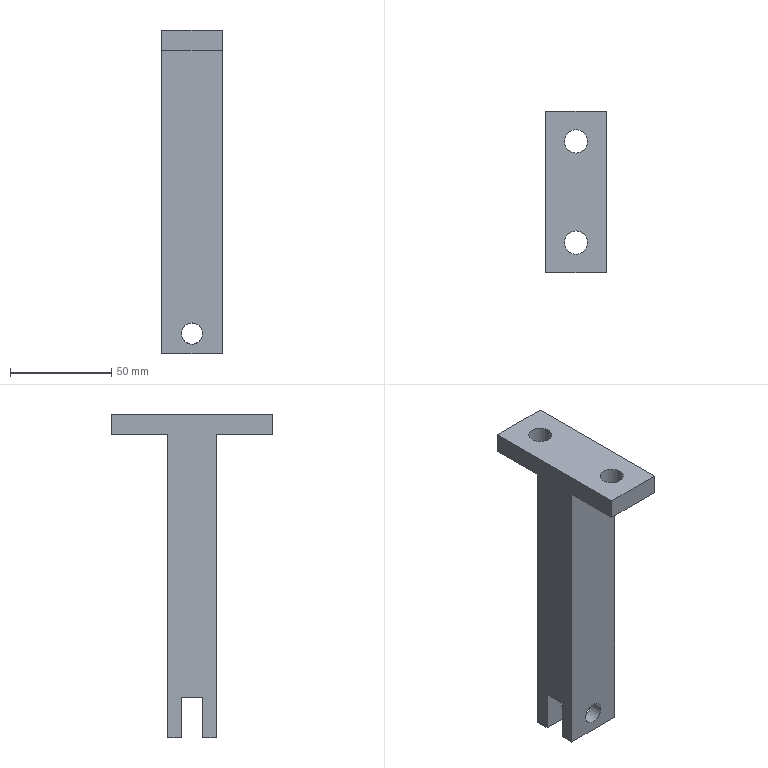Part | NX | features solid 2 | 1 solid | 19 faces | box 30 x 80 x 160 mm | volume 112089 mm3 | plane 15 | cylinder 4 | commonest cylinder face diameters 10.5 x2 11.5 x2
STEP:
#1=CARTESIAN_POINT('',(-925.,73.,-134.));
#2=VERTEX_POINT('',#1);
#3=CARTESIAN_POINT('',(-925.,79.75,-134.));
#4=VERTEX_POINT('',#3);
#5=CARTESIAN_POINT('',(-925.,73.,-134.));
#6=DIRECTION('',(0.,1.,0.));
#7=VECTOR('',#6,1000.);
#8=LINE('',#5,#7);
#9=EDGE_CURVE('',#2,#4,#8,.T.);
#10=ORIENTED_EDGE('',*,*,#9,.T.);
#11=CARTESIAN_POINT('',(-895.,79.75,-134.));
#12=VERTEX_POINT('',#11);
#13=CARTESIAN_POINT('',(-895.,79.75,-134.));
#14=DIRECTION('',(-1.,0.,0.));
#15=VECTOR('',#14,1000.);
#16=LINE('',#13,#15);
#17=EDGE_CURVE('',#12,#4,#16,.T.);
#18=ORIENTED_EDGE('',*,*,#17,.F.);
#19=CARTESIAN_POINT('',(-895.,73.,-134.));
#20=VERTEX_POINT('',#19);
#21=CARTESIAN_POINT('',(-895.,97.,-134.));
#22=DIRECTION('',(0.,-1.,0.));
#23=VECTOR('',#22,1000.);
#24=LINE('',#21,#23);
#25=EDGE_CURVE('',#12,#20,#24,.T.);
#26=ORIENTED_EDGE('',*,*,#25,.T.);
#27=CARTESIAN_POINT('',(-895.,73.,-134.));
#28=DIRECTION('',(-1.,0.,0.));
#29=VECTOR('',#28,1000.);
#30=LINE('',#27,#29);
#31=EDGE_CURVE('',#20,#2,#30,.T.);
#32=ORIENTED_EDGE('',*,*,#31,.T.);
#33=EDGE_LOOP('',(#10,#18,#26,#32));
#34=FACE_BOUND('',#33,.T.);
#35=CARTESIAN_POINT('',(-925.,73.,-134.));
#36=DIRECTION('',(0.,0.,1.));
#37=DIRECTION('',(0.,1.,0.));
#38=AXIS2_PLACEMENT_3D('',#35,#36,#37);
#39=PLANE('',#38);
#40=ADVANCED_FACE('',(#34),#39,.F.);
#41=CARTESIAN_POINT('',(-925.,79.75,-114.));
#42=VERTEX_POINT('',#41);
#43=CARTESIAN_POINT('',(-925.,79.75,-114.));
#44=DIRECTION('',(0.,0.,-1.));
#45=VECTOR('',#44,1000.);
#46=LINE('',#43,#45);
#47=EDGE_CURVE('',#42,#4,#46,.T.);
#48=ORIENTED_EDGE('',*,*,#47,.T.);
#49=ORIENTED_EDGE('',*,*,#9,.F.);
#50=CARTESIAN_POINT('',(-925.,73.,16.));
#51=VERTEX_POINT('',#50);
#52=CARTESIAN_POINT('',(-925.,73.,26.));
#53=DIRECTION('',(0.,0.,-1.));
#54=VECTOR('',#53,1000.);
#55=LINE('',#52,#54);
#56=EDGE_CURVE('',#51,#2,#55,.T.);
#57=ORIENTED_EDGE('',*,*,#56,.F.);
#58=CARTESIAN_POINT('',(-925.,45.,16.));
#59=VERTEX_POINT('',#58);
#60=CARTESIAN_POINT('',(-925.,45.,16.));
#61=DIRECTION('',(0.,1.,0.));
#62=VECTOR('',#61,1000.);
#63=LINE('',#60,#62);
#64=EDGE_CURVE('',#59,#51,#63,.T.);
#65=ORIENTED_EDGE('',*,*,#64,.F.);
#66=CARTESIAN_POINT('',(-925.,45.,26.));
#67=VERTEX_POINT('',#66);
#68=CARTESIAN_POINT('',(-925.,45.,26.));
#69=DIRECTION('',(0.,0.,-1.));
#70=VECTOR('',#69,1000.);
#71=LINE('',#68,#70);
#72=EDGE_CURVE('',#67,#59,#71,.T.);
#73=ORIENTED_EDGE('',*,*,#72,.F.);
#74=CARTESIAN_POINT('',(-925.,125.,26.));
#75=VERTEX_POINT('',#74);
#76=CARTESIAN_POINT('',(-925.,73.,26.));
#77=DIRECTION('',(0.,1.,0.));
#78=VECTOR('',#77,1000.);
#79=LINE('',#76,#78);
#80=EDGE_CURVE('',#67,#75,#79,.T.);
#81=ORIENTED_EDGE('',*,*,#80,.T.);
#82=CARTESIAN_POINT('',(-925.,125.,16.));
#83=VERTEX_POINT('',#82);
#84=CARTESIAN_POINT('',(-925.,125.,26.));
#85=DIRECTION('',(0.,0.,-1.));
#86=VECTOR('',#85,1000.);
#87=LINE('',#84,#86);
#88=EDGE_CURVE('',#75,#83,#87,.T.);
#89=ORIENTED_EDGE('',*,*,#88,.T.);
#90=CARTESIAN_POINT('',(-925.,97.,16.));
#91=VERTEX_POINT('',#90);
#92=CARTESIAN_POINT('',(-925.,45.,16.));
#93=DIRECTION('',(0.,1.,0.));
#94=VECTOR('',#93,1000.);
#95=LINE('',#92,#94);
#96=EDGE_CURVE('',#91,#83,#95,.T.);
#97=ORIENTED_EDGE('',*,*,#96,.F.);
#98=CARTESIAN_POINT('',(-925.,97.,-134.));
#99=VERTEX_POINT('',#98);
#100=CARTESIAN_POINT('',(-925.,97.,26.));
#101=DIRECTION('',(0.,0.,-1.));
#102=VECTOR('',#101,1000.);
#103=LINE('',#100,#102);
#104=EDGE_CURVE('',#91,#99,#103,.T.);
#105=ORIENTED_EDGE('',*,*,#104,.T.);
#106=CARTESIAN_POINT('',(-925.,90.25,-134.));
#107=VERTEX_POINT('',#106);
#108=CARTESIAN_POINT('',(-925.,73.,-134.));
#109=DIRECTION('',(0.,1.,0.));
#110=VECTOR('',#109,1000.);
#111=LINE('',#108,#110);
#112=EDGE_CURVE('',#107,#99,#111,.T.);
#113=ORIENTED_EDGE('',*,*,#112,.F.);
#114=CARTESIAN_POINT('',(-925.,90.25,-114.));
#115=VERTEX_POINT('',#114);
#116=CARTESIAN_POINT('',(-925.,90.25,-114.));
#117=DIRECTION('',(0.,0.,-1.));
#118=VECTOR('',#117,1000.);
#119=LINE('',#116,#118);
#120=EDGE_CURVE('',#115,#107,#119,.T.);
#121=ORIENTED_EDGE('',*,*,#120,.F.);
#122=CARTESIAN_POINT('',(-925.,79.75,-114.));
#123=DIRECTION('',(0.,1.,0.));
#124=VECTOR('',#123,1000.);
#125=LINE('',#122,#124);
#126=EDGE_CURVE('',#42,#115,#125,.T.);
#127=ORIENTED_EDGE('',*,*,#126,.F.);
#128=EDGE_LOOP('',(#48,#49,#57,#65,#73,#81,#89,#97,#105,#113,#121,#127));
#129=FACE_BOUND('',#128,.T.);
#130=CARTESIAN_POINT('',(-925.,73.,26.));
#131=DIRECTION('',(-1.,0.,0.));
#132=DIRECTION('',(0.,0.,1.));
#133=AXIS2_PLACEMENT_3D('',#130,#131,#132);
#134=PLANE('',#133);
#135=ADVANCED_FACE('',(#129),#134,.T.);
#136=CARTESIAN_POINT('',(-915.25,97.,-124.));
#137=VERTEX_POINT('',#136);
#138=CARTESIAN_POINT('',(-910.,97.,-124.));
#139=DIRECTION('',(0.,1.,0.));
#140=DIRECTION('',(-1.,0.,0.));
#141=AXIS2_PLACEMENT_3D('',#138,#139,#140);
#142=CIRCLE('',#141,5.25);
#143=EDGE_CURVE('',#137,#137,#142,.T.);
#144=ORIENTED_EDGE('',*,*,#143,.F.);
#145=EDGE_LOOP('',(#144));
#146=FACE_BOUND('',#145,.T.);
#147=CARTESIAN_POINT('',(-895.,97.,16.));
#148=VERTEX_POINT('',#147);
#149=CARTESIAN_POINT('',(-925.,97.,16.));
#150=DIRECTION('',(-1.,0.,0.));
#151=VECTOR('',#150,1000.);
#152=LINE('',#149,#151);
#153=EDGE_CURVE('',#148,#91,#152,.T.);
#154=ORIENTED_EDGE('',*,*,#153,.F.);
#155=CARTESIAN_POINT('',(-895.,97.,-134.));
#156=VERTEX_POINT('',#155);
#157=CARTESIAN_POINT('',(-895.,97.,26.));
#158=DIRECTION('',(0.,0.,-1.));
#159=VECTOR('',#158,1000.);
#160=LINE('',#157,#159);
#161=EDGE_CURVE('',#148,#156,#160,.T.);
#162=ORIENTED_EDGE('',*,*,#161,.T.);
#163=CARTESIAN_POINT('',(-925.,97.,-134.));
#164=DIRECTION('',(1.,0.,0.));
#165=VECTOR('',#164,1000.);
#166=LINE('',#163,#165);
#167=EDGE_CURVE('',#99,#156,#166,.T.);
#168=ORIENTED_EDGE('',*,*,#167,.F.);
#169=ORIENTED_EDGE('',*,*,#104,.F.);
#170=EDGE_LOOP('',(#154,#162,#168,#169));
#171=FACE_BOUND('',#170,.T.);
#172=CARTESIAN_POINT('',(-925.,97.,26.));
#173=DIRECTION('',(0.,1.,0.));
#174=DIRECTION('',(-1.,0.,0.));
#175=AXIS2_PLACEMENT_3D('',#172,#173,#174);
#176=PLANE('',#175);
#177=ADVANCED_FACE('',(#146,#171),#176,.T.);
#178=CARTESIAN_POINT('',(-895.,79.75,-28.163));
#179=VERTEX_POINT('',#178);
#180=CARTESIAN_POINT('',(-895.,79.75,-114.));
#181=DIRECTION('',(0.,0.,-1.));
#182=VECTOR('',#181,1000.);
#183=LINE('',#180,#182);
#184=EDGE_CURVE('',#179,#12,#183,.T.);
#185=ORIENTED_EDGE('',*,*,#184,.F.);
#186=CARTESIAN_POINT('',(-895.,90.25,-28.163));
#187=VERTEX_POINT('',#186);
#188=CARTESIAN_POINT('',(-895.,97.,-28.163));
#189=DIRECTION('',(0.,1.,0.));
#190=VECTOR('',#189,1000.);
#191=LINE('',#188,#190);
#192=EDGE_CURVE('',#179,#187,#191,.T.);
#193=ORIENTED_EDGE('',*,*,#192,.T.);
#194=CARTESIAN_POINT('',(-895.,90.25,-134.));
#195=VERTEX_POINT('',#194);
#196=CARTESIAN_POINT('',(-895.,90.25,-114.));
#197=DIRECTION('',(0.,0.,-1.));
#198=VECTOR('',#197,1000.);
#199=LINE('',#196,#198);
#200=EDGE_CURVE('',#187,#195,#199,.T.);
#201=ORIENTED_EDGE('',*,*,#200,.T.);
#202=CARTESIAN_POINT('',(-895.,97.,-134.));
#203=DIRECTION('',(0.,-1.,0.));
#204=VECTOR('',#203,1000.);
#205=LINE('',#202,#204);
#206=EDGE_CURVE('',#156,#195,#205,.T.);
#207=ORIENTED_EDGE('',*,*,#206,.F.);
#208=ORIENTED_EDGE('',*,*,#161,.F.);
#209=CARTESIAN_POINT('',(-895.,125.,16.));
#210=VERTEX_POINT('',#209);
#211=CARTESIAN_POINT('',(-895.,125.,16.));
#212=DIRECTION('',(0.,-1.,0.));
#213=VECTOR('',#212,1000.);
#214=LINE('',#211,#213);
#215=EDGE_CURVE('',#210,#148,#214,.T.);
#216=ORIENTED_EDGE('',*,*,#215,.F.);
#217=CARTESIAN_POINT('',(-895.,125.,26.));
#218=VERTEX_POINT('',#217);
#219=CARTESIAN_POINT('',(-895.,125.,26.));
#220=DIRECTION('',(0.,0.,-1.));
#221=VECTOR('',#220,1000.);
#222=LINE('',#219,#221);
#223=EDGE_CURVE('',#218,#210,#222,.T.);
#224=ORIENTED_EDGE('',*,*,#223,.F.);
#225=CARTESIAN_POINT('',(-895.,45.,26.));
#226=VERTEX_POINT('',#225);
#227=CARTESIAN_POINT('',(-895.,97.,26.));
#228=DIRECTION('',(0.,-1.,0.));
#229=VECTOR('',#228,1000.);
#230=LINE('',#227,#229);
#231=EDGE_CURVE('',#218,#226,#230,.T.);
#232=ORIENTED_EDGE('',*,*,#231,.T.);
#233=CARTESIAN_POINT('',(-895.,45.,16.));
#234=VERTEX_POINT('',#233);
#235=CARTESIAN_POINT('',(-895.,45.,26.));
#236=DIRECTION('',(0.,0.,-1.));
#237=VECTOR('',#236,1000.);
#238=LINE('',#235,#237);
#239=EDGE_CURVE('',#226,#234,#238,.T.);
#240=ORIENTED_EDGE('',*,*,#239,.T.);
#241=CARTESIAN_POINT('',(-895.,73.,16.));
#242=VERTEX_POINT('',#241);
#243=CARTESIAN_POINT('',(-895.,125.,16.));
#244=DIRECTION('',(0.,-1.,0.));
#245=VECTOR('',#244,1000.);
#246=LINE('',#243,#245);
#247=EDGE_CURVE('',#242,#234,#246,.T.);
#248=ORIENTED_EDGE('',*,*,#247,.F.);
#249=CARTESIAN_POINT('',(-895.,73.,26.));
#250=DIRECTION('',(0.,0.,-1.));
#251=VECTOR('',#250,1000.);
#252=LINE('',#249,#251);
#253=EDGE_CURVE('',#242,#20,#252,.T.);
#254=ORIENTED_EDGE('',*,*,#253,.T.);
#255=ORIENTED_EDGE('',*,*,#25,.F.);
#256=EDGE_LOOP('',(#185,#193,#201,#207,#208,#216,#224,#232,#240,#248,#254,#255));
#257=FACE_BOUND('',#256,.T.);
#258=CARTESIAN_POINT('',(-895.,97.,26.));
#259=DIRECTION('',(1.,0.,0.));
#260=DIRECTION('',(0.,1.,0.));
#261=AXIS2_PLACEMENT_3D('',#258,#259,#260);
#262=PLANE('',#261);
#263=ADVANCED_FACE('',(#257),#262,.T.);
#264=CARTESIAN_POINT('',(-910.,73.,-129.25));
#265=VERTEX_POINT('',#264);
#266=CARTESIAN_POINT('',(-910.,73.,-124.));
#267=DIRECTION('',(0.,1.,0.));
#268=DIRECTION('',(0.,0.,-1.));
#269=AXIS2_PLACEMENT_3D('',#266,#267,#268);
#270=CIRCLE('',#269,5.25);
#271=EDGE_CURVE('',#265,#265,#270,.T.);
#272=ORIENTED_EDGE('',*,*,#271,.T.);
#273=EDGE_LOOP('',(#272));
#274=FACE_BOUND('',#273,.T.);
#275=CARTESIAN_POINT('',(-895.,73.,16.));
#276=DIRECTION('',(1.,0.,0.));
#277=VECTOR('',#276,1000.);
#278=LINE('',#275,#277);
#279=EDGE_CURVE('',#51,#242,#278,.T.);
#280=ORIENTED_EDGE('',*,*,#279,.F.);
#281=ORIENTED_EDGE('',*,*,#56,.T.);
#282=ORIENTED_EDGE('',*,*,#31,.F.);
#283=ORIENTED_EDGE('',*,*,#253,.F.);
#284=EDGE_LOOP('',(#280,#281,#282,#283));
#285=FACE_BOUND('',#284,.T.);
#286=CARTESIAN_POINT('',(-895.,73.,26.));
#287=DIRECTION('',(0.,-1.,0.));
#288=DIRECTION('',(0.,0.,1.));
#289=AXIS2_PLACEMENT_3D('',#286,#287,#288);
#290=PLANE('',#289);
#291=ADVANCED_FACE('',(#274,#285),#290,.T.);
#292=CARTESIAN_POINT('',(-910.,54.25,26.));
#293=VERTEX_POINT('',#292);
#294=CARTESIAN_POINT('',(-910.,60.,26.));
#295=DIRECTION('',(0.,0.,-1.));
#296=DIRECTION('',(0.,-1.,0.));
#297=AXIS2_PLACEMENT_3D('',#294,#295,#296);
#298=CIRCLE('',#297,5.75);
#299=EDGE_CURVE('',#293,#293,#298,.T.);
#300=ORIENTED_EDGE('',*,*,#299,.T.);
#301=EDGE_LOOP('',(#300));
#302=FACE_BOUND('',#301,.T.);
#303=CARTESIAN_POINT('',(-910.,104.25,26.));
#304=VERTEX_POINT('',#303);
#305=CARTESIAN_POINT('',(-910.,110.,26.));
#306=DIRECTION('',(0.,0.,-1.));
#307=DIRECTION('',(0.,-1.,0.));
#308=AXIS2_PLACEMENT_3D('',#305,#306,#307);
#309=CIRCLE('',#308,5.75);
#310=EDGE_CURVE('',#304,#304,#309,.T.);
#311=ORIENTED_EDGE('',*,*,#310,.T.);
#312=EDGE_LOOP('',(#311));
#313=FACE_BOUND('',#312,.T.);
#314=ORIENTED_EDGE('',*,*,#80,.F.);
#315=CARTESIAN_POINT('',(-895.,45.,26.));
#316=DIRECTION('',(-1.,0.,0.));
#317=VECTOR('',#316,1000.);
#318=LINE('',#315,#317);
#319=EDGE_CURVE('',#226,#67,#318,.T.);
#320=ORIENTED_EDGE('',*,*,#319,.F.);
#321=ORIENTED_EDGE('',*,*,#231,.F.);
#322=CARTESIAN_POINT('',(-925.,125.,26.));
#323=DIRECTION('',(1.,0.,0.));
#324=VECTOR('',#323,1000.);
#325=LINE('',#322,#324);
#326=EDGE_CURVE('',#75,#218,#325,.T.);
#327=ORIENTED_EDGE('',*,*,#326,.F.);
#328=EDGE_LOOP('',(#314,#320,#321,#327));
#329=FACE_BOUND('',#328,.T.);
#330=CARTESIAN_POINT('',(-925.,73.,26.));
#331=DIRECTION('',(0.,0.,1.));
#332=DIRECTION('',(0.,1.,0.));
#333=AXIS2_PLACEMENT_3D('',#330,#331,#332);
#334=PLANE('',#333);
#335=ADVANCED_FACE('',(#302,#313,#329),#334,.T.);
#336=ORIENTED_EDGE('',*,*,#206,.T.);
#337=CARTESIAN_POINT('',(-925.,90.25,-134.));
#338=DIRECTION('',(1.,0.,0.));
#339=VECTOR('',#338,1000.);
#340=LINE('',#337,#339);
#341=EDGE_CURVE('',#107,#195,#340,.T.);
#342=ORIENTED_EDGE('',*,*,#341,.F.);
#343=ORIENTED_EDGE('',*,*,#112,.T.);
#344=ORIENTED_EDGE('',*,*,#167,.T.);
#345=EDGE_LOOP('',(#336,#342,#343,#344));
#346=FACE_BOUND('',#345,.T.);
#347=CARTESIAN_POINT('',(-925.,73.,-134.));
#348=DIRECTION('',(0.,0.,1.));
#349=DIRECTION('',(0.,1.,0.));
#350=AXIS2_PLACEMENT_3D('',#347,#348,#349);
#351=PLANE('',#350);
#352=ADVANCED_FACE('',(#346),#351,.F.);
#353=CARTESIAN_POINT('',(-895.,45.,16.));
#354=DIRECTION('',(-1.,0.,0.));
#355=VECTOR('',#354,1000.);
#356=LINE('',#353,#355);
#357=EDGE_CURVE('',#234,#59,#356,.T.);
#358=ORIENTED_EDGE('',*,*,#357,.F.);
#359=ORIENTED_EDGE('',*,*,#239,.F.);
#360=ORIENTED_EDGE('',*,*,#319,.T.);
#361=ORIENTED_EDGE('',*,*,#72,.T.);
#362=EDGE_LOOP('',(#358,#359,#360,#361));
#363=FACE_BOUND('',#362,.T.);
#364=CARTESIAN_POINT('',(-895.,45.,26.));
#365=DIRECTION('',(0.,-1.,0.));
#366=DIRECTION('',(0.,0.,1.));
#367=AXIS2_PLACEMENT_3D('',#364,#365,#366);
#368=PLANE('',#367);
#369=ADVANCED_FACE('',(#363),#368,.T.);
#370=CARTESIAN_POINT('',(-910.,54.25,16.));
#371=VERTEX_POINT('',#370);
#372=CARTESIAN_POINT('',(-910.,60.,16.));
#373=DIRECTION('',(0.,0.,-1.));
#374=DIRECTION('',(0.,-1.,0.));
#375=AXIS2_PLACEMENT_3D('',#372,#373,#374);
#376=CIRCLE('',#375,5.75);
#377=EDGE_CURVE('',#371,#371,#376,.T.);
#378=ORIENTED_EDGE('',*,*,#377,.F.);
#379=EDGE_LOOP('',(#378));
#380=FACE_BOUND('',#379,.T.);
#381=ORIENTED_EDGE('',*,*,#64,.T.);
#382=ORIENTED_EDGE('',*,*,#279,.T.);
#383=ORIENTED_EDGE('',*,*,#247,.T.);
#384=ORIENTED_EDGE('',*,*,#357,.T.);
#385=EDGE_LOOP('',(#381,#382,#383,#384));
#386=FACE_BOUND('',#385,.T.);
#387=CARTESIAN_POINT('',(-925.,125.,16.));
#388=DIRECTION('',(0.,0.,-1.));
#389=DIRECTION('',(0.,-1.,0.));
#390=AXIS2_PLACEMENT_3D('',#387,#388,#389);
#391=PLANE('',#390);
#392=ADVANCED_FACE('',(#380,#386),#391,.T.);
#393=CARTESIAN_POINT('',(-910.,104.25,16.));
#394=VERTEX_POINT('',#393);
#395=CARTESIAN_POINT('',(-910.,110.,16.));
#396=DIRECTION('',(0.,0.,-1.));
#397=DIRECTION('',(0.,-1.,0.));
#398=AXIS2_PLACEMENT_3D('',#395,#396,#397);
#399=CIRCLE('',#398,5.75);
#400=EDGE_CURVE('',#394,#394,#399,.T.);
#401=ORIENTED_EDGE('',*,*,#400,.F.);
#402=EDGE_LOOP('',(#401));
#403=FACE_BOUND('',#402,.T.);
#404=ORIENTED_EDGE('',*,*,#215,.T.);
#405=ORIENTED_EDGE('',*,*,#153,.T.);
#406=ORIENTED_EDGE('',*,*,#96,.T.);
#407=CARTESIAN_POINT('',(-925.,125.,16.));
#408=DIRECTION('',(1.,0.,0.));
#409=VECTOR('',#408,1000.);
#410=LINE('',#407,#409);
#411=EDGE_CURVE('',#83,#210,#410,.T.);
#412=ORIENTED_EDGE('',*,*,#411,.T.);
#413=EDGE_LOOP('',(#404,#405,#406,#412));
#414=FACE_BOUND('',#413,.T.);
#415=CARTESIAN_POINT('',(-925.,125.,16.));
#416=DIRECTION('',(0.,0.,-1.));
#417=DIRECTION('',(0.,-1.,0.));
#418=AXIS2_PLACEMENT_3D('',#415,#416,#417);
#419=PLANE('',#418);
#420=ADVANCED_FACE('',(#403,#414),#419,.T.);
#421=ORIENTED_EDGE('',*,*,#411,.F.);
#422=ORIENTED_EDGE('',*,*,#88,.F.);
#423=ORIENTED_EDGE('',*,*,#326,.T.);
#424=ORIENTED_EDGE('',*,*,#223,.T.);
#425=EDGE_LOOP('',(#421,#422,#423,#424));
#426=FACE_BOUND('',#425,.T.);
#427=CARTESIAN_POINT('',(-925.,125.,26.));
#428=DIRECTION('',(0.,1.,0.));
#429=DIRECTION('',(0.,0.,-1.));
#430=AXIS2_PLACEMENT_3D('',#427,#428,#429);
#431=PLANE('',#430);
#432=ADVANCED_FACE('',(#426),#431,.T.);
#433=CARTESIAN_POINT('',(-910.,79.75,-118.75));
#434=VERTEX_POINT('',#433);
#435=CARTESIAN_POINT('',(-910.,79.75,-124.));
#436=DIRECTION('',(0.,-1.,0.));
#437=DIRECTION('',(0.,0.,1.));
#438=AXIS2_PLACEMENT_3D('',#435,#436,#437);
#439=CIRCLE('',#438,5.25);
#440=EDGE_CURVE('',#434,#434,#439,.T.);
#441=ORIENTED_EDGE('',*,*,#440,.T.);
#442=EDGE_LOOP('',(#441));
#443=FACE_BOUND('',#442,.T.);
#444=ORIENTED_EDGE('',*,*,#17,.T.);
#445=ORIENTED_EDGE('',*,*,#47,.F.);
#446=CARTESIAN_POINT('',(-918.,79.75,-114.));
#447=VERTEX_POINT('',#446);
#448=CARTESIAN_POINT('',(-895.,79.75,-114.));
#449=DIRECTION('',(-1.,0.,0.));
#450=VECTOR('',#449,1000.);
#451=LINE('',#448,#450);
#452=EDGE_CURVE('',#447,#42,#451,.T.);
#453=ORIENTED_EDGE('',*,*,#452,.F.);
#454=CARTESIAN_POINT('',(-916.459,79.75,-108.25));
#455=DIRECTION('',(-0.2588,0.,-0.9659));
#456=VECTOR('',#455,1000.);
#457=LINE('',#454,#456);
#458=EDGE_CURVE('',#447,#179,#457,.F.);
#459=ORIENTED_EDGE('',*,*,#458,.T.);
#460=ORIENTED_EDGE('',*,*,#184,.T.);
#461=EDGE_LOOP('',(#444,#445,#453,#459,#460));
#462=FACE_BOUND('',#461,.T.);
#463=CARTESIAN_POINT('',(-895.,79.75,-114.));
#464=DIRECTION('',(0.,-1.,0.));
#465=DIRECTION('',(0.,0.,1.));
#466=AXIS2_PLACEMENT_3D('',#463,#464,#465);
#467=PLANE('',#466);
#468=ADVANCED_FACE('',(#443,#462),#467,.F.);
#469=CARTESIAN_POINT('',(-915.25,90.25,-124.));
#470=VERTEX_POINT('',#469);
#471=CARTESIAN_POINT('',(-910.,90.25,-124.));
#472=DIRECTION('',(0.,1.,0.));
#473=DIRECTION('',(-1.,0.,0.));
#474=AXIS2_PLACEMENT_3D('',#471,#472,#473);
#475=CIRCLE('',#474,5.25);
#476=EDGE_CURVE('',#470,#470,#475,.T.);
#477=ORIENTED_EDGE('',*,*,#476,.T.);
#478=EDGE_LOOP('',(#477));
#479=FACE_BOUND('',#478,.T.);
#480=ORIENTED_EDGE('',*,*,#341,.T.);
#481=ORIENTED_EDGE('',*,*,#200,.F.);
#482=CARTESIAN_POINT('',(-918.,90.25,-114.));
#483=VERTEX_POINT('',#482);
#484=CARTESIAN_POINT('',(-918.469,90.25,-115.75));
#485=DIRECTION('',(0.2588,0.,0.9659));
#486=VECTOR('',#485,1000.);
#487=LINE('',#484,#486);
#488=EDGE_CURVE('',#187,#483,#487,.F.);
#489=ORIENTED_EDGE('',*,*,#488,.T.);
#490=CARTESIAN_POINT('',(-925.,90.25,-114.));
#491=DIRECTION('',(1.,0.,0.));
#492=VECTOR('',#491,1000.);
#493=LINE('',#490,#492);
#494=EDGE_CURVE('',#115,#483,#493,.T.);
#495=ORIENTED_EDGE('',*,*,#494,.F.);
#496=ORIENTED_EDGE('',*,*,#120,.T.);
#497=EDGE_LOOP('',(#480,#481,#489,#495,#496));
#498=FACE_BOUND('',#497,.T.);
#499=CARTESIAN_POINT('',(-925.,90.25,-114.));
#500=DIRECTION('',(0.,1.,0.));
#501=DIRECTION('',(-1.,0.,0.));
#502=AXIS2_PLACEMENT_3D('',#499,#500,#501);
#503=PLANE('',#502);
#504=ADVANCED_FACE('',(#479,#498),#503,.F.);
#505=ORIENTED_EDGE('',*,*,#494,.T.);
#506=CARTESIAN_POINT('',(-918.,79.75,-114.));
#507=DIRECTION('',(0.,-1.,0.));
#508=VECTOR('',#507,1000.);
#509=LINE('',#506,#508);
#510=EDGE_CURVE('',#483,#447,#509,.T.);
#511=ORIENTED_EDGE('',*,*,#510,.T.);
#512=ORIENTED_EDGE('',*,*,#452,.T.);
#513=ORIENTED_EDGE('',*,*,#126,.T.);
#514=EDGE_LOOP('',(#505,#511,#512,#513));
#515=FACE_BOUND('',#514,.T.);
#516=CARTESIAN_POINT('',(-895.,79.75,-114.));
#517=DIRECTION('',(0.,0.,-1.));
#518=DIRECTION('',(0.,-1.,0.));
#519=AXIS2_PLACEMENT_3D('',#516,#517,#518);
#520=PLANE('',#519);
#521=ADVANCED_FACE('',(#515),#520,.T.);
#522=ORIENTED_EDGE('',*,*,#488,.F.);
#523=ORIENTED_EDGE('',*,*,#192,.F.);
#524=ORIENTED_EDGE('',*,*,#458,.F.);
#525=ORIENTED_EDGE('',*,*,#510,.F.);
#526=EDGE_LOOP('',(#522,#523,#524,#525));
#527=FACE_BOUND('',#526,.T.);
#528=CARTESIAN_POINT('',(-918.,79.75,-114.));
#529=DIRECTION('',(-0.9659,0.,0.2588));
#530=DIRECTION('',(0.2588,0.,0.9659));
#531=AXIS2_PLACEMENT_3D('',#528,#529,#530);
#532=PLANE('',#531);
#533=ADVANCED_FACE('',(#527),#532,.F.);
#534=ORIENTED_EDGE('',*,*,#143,.T.);
#535=EDGE_LOOP('',(#534));
#536=FACE_BOUND('',#535,.T.);
#537=ORIENTED_EDGE('',*,*,#476,.F.);
#538=EDGE_LOOP('',(#537));
#539=FACE_BOUND('',#538,.T.);
#540=CARTESIAN_POINT('',(-910.,73.,-124.));
#541=DIRECTION('',(0.,1.,0.));
#542=DIRECTION('',(0.,0.,-1.));
#543=AXIS2_PLACEMENT_3D('',#540,#541,#542);
#544=CYLINDRICAL_SURFACE('',#543,5.25);
#545=ADVANCED_FACE('',(#536,#539),#544,.F.);
#546=ORIENTED_EDGE('',*,*,#271,.F.);
#547=EDGE_LOOP('',(#546));
#548=FACE_BOUND('',#547,.T.);
#549=ORIENTED_EDGE('',*,*,#440,.F.);
#550=EDGE_LOOP('',(#549));
#551=FACE_BOUND('',#550,.T.);
#552=CARTESIAN_POINT('',(-910.,73.,-124.));
#553=DIRECTION('',(0.,1.,0.));
#554=DIRECTION('',(0.,0.,-1.));
#555=AXIS2_PLACEMENT_3D('',#552,#553,#554);
#556=CYLINDRICAL_SURFACE('',#555,5.25);
#557=ADVANCED_FACE('',(#548,#551),#556,.F.);
#558=ORIENTED_EDGE('',*,*,#400,.T.);
#559=EDGE_LOOP('',(#558));
#560=FACE_BOUND('',#559,.T.);
#561=ORIENTED_EDGE('',*,*,#310,.F.);
#562=EDGE_LOOP('',(#561));
#563=FACE_BOUND('',#562,.T.);
#564=CARTESIAN_POINT('',(-910.,110.,26.));
#565=DIRECTION('',(0.,0.,-1.));
#566=DIRECTION('',(0.,-1.,0.));
#567=AXIS2_PLACEMENT_3D('',#564,#565,#566);
#568=CYLINDRICAL_SURFACE('',#567,5.75);
#569=ADVANCED_FACE('',(#560,#563),#568,.F.);
#570=ORIENTED_EDGE('',*,*,#377,.T.);
#571=EDGE_LOOP('',(#570));
#572=FACE_BOUND('',#571,.T.);
#573=ORIENTED_EDGE('',*,*,#299,.F.);
#574=EDGE_LOOP('',(#573));
#575=FACE_BOUND('',#574,.T.);
#576=CARTESIAN_POINT('',(-910.,60.,26.));
#577=DIRECTION('',(0.,0.,-1.));
#578=DIRECTION('',(0.,-1.,0.));
#579=AXIS2_PLACEMENT_3D('',#576,#577,#578);
#580=CYLINDRICAL_SURFACE('',#579,5.75);
#581=ADVANCED_FACE('',(#572,#575),#580,.F.);
#582=CLOSED_SHELL('',(#40,#135,#177,#263,#291,#335,#352,#369,#392,#420,#432,#468,#504,#521,#533,#545,#557,#569,#581));
#583=MANIFOLD_SOLID_BREP('',#582);
#584=(LENGTH_UNIT()NAMED_UNIT(*)SI_UNIT(.MILLI.,.METRE.));
#585=UNCERTAINTY_MEASURE_WITH_UNIT(LENGTH_MEASURE(0.00001),#584,'','');
#586=(NAMED_UNIT(*)PLANE_ANGLE_UNIT()SI_UNIT($,.RADIAN.));
#587=(NAMED_UNIT(*)SI_UNIT($,.STERADIAN.)SOLID_ANGLE_UNIT());
#588=(GEOMETRIC_REPRESENTATION_CONTEXT(3)GLOBAL_UNCERTAINTY_ASSIGNED_CONTEXT((#585))GLOBAL_UNIT_ASSIGNED_CONTEXT((#584,#586,#587))REPRESENTATION_CONTEXT('',''));
#589=ADVANCED_BREP_SHAPE_REPRESENTATION('',(#583),#588);